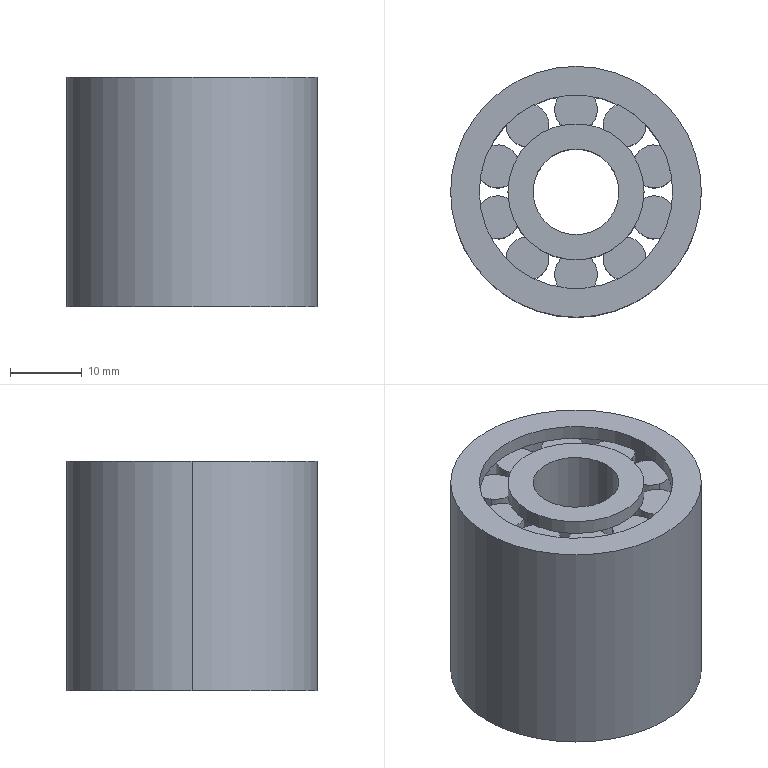Part | NX | features BREP 12 | 12 solids | 64 faces | box 35 x 35 x 32 mm | volume 21762 mm3 | cylinder 36 | plane 28 | commonest cylinder face diameters 6 x20 19 x4 27 x4 12 x2 17 x2 29 x2
STEP:
#1=CARTESIAN_POINT('',(-11.864,-0.7005,29.95));
#2=VERTEX_POINT('',#1);
#3=CARTESIAN_POINT('',(-10.01,-6.407,29.95));
#4=VERTEX_POINT('',#3);
#5=CARTESIAN_POINT('',(-10.937,-3.554,29.95));
#6=DIRECTION('',(0.,0.,1.));
#7=DIRECTION('',(-0.309,0.9511,0.));
#8=AXIS2_PLACEMENT_3D('',#5,#6,#7);
#9=CIRCLE('',#8,3.);
#10=EDGE_CURVE('',#2,#4,#9,.T.);
#11=ORIENTED_EDGE('',*,*,#10,.F.);
#12=CARTESIAN_POINT('',(-11.864,-0.7005,2.05));
#13=VERTEX_POINT('',#12);
#14=CARTESIAN_POINT('',(-11.864,-0.7005,29.95));
#15=DIRECTION('',(0.,0.,-1.));
#16=VECTOR('',#15,1000.);
#17=LINE('',#14,#16);
#18=EDGE_CURVE('',#2,#13,#17,.T.);
#19=ORIENTED_EDGE('',*,*,#18,.T.);
#20=CARTESIAN_POINT('',(-10.01,-6.407,2.05));
#21=VERTEX_POINT('',#20);
#22=CARTESIAN_POINT('',(-10.937,-3.554,2.05));
#23=DIRECTION('',(0.,0.,1.));
#24=DIRECTION('',(-0.309,0.9511,0.));
#25=AXIS2_PLACEMENT_3D('',#22,#23,#24);
#26=CIRCLE('',#25,3.);
#27=EDGE_CURVE('',#13,#21,#26,.T.);
#28=ORIENTED_EDGE('',*,*,#27,.T.);
#29=CARTESIAN_POINT('',(-10.01,-6.407,29.95));
#30=DIRECTION('',(0.,0.,-1.));
#31=VECTOR('',#30,1000.);
#32=LINE('',#29,#31);
#33=EDGE_CURVE('',#4,#21,#32,.T.);
#34=ORIENTED_EDGE('',*,*,#33,.F.);
#35=EDGE_LOOP('',(#11,#19,#28,#34));
#36=FACE_BOUND('',#35,.T.);
#37=CARTESIAN_POINT('',(-10.937,-3.554,29.95));
#38=DIRECTION('',(0.,0.,-1.));
#39=DIRECTION('',(-0.309,0.9511,0.));
#40=AXIS2_PLACEMENT_3D('',#37,#38,#39);
#41=CYLINDRICAL_SURFACE('',#40,3.);
#42=ADVANCED_FACE('',(#36),#41,.T.);
#43=ORIENTED_EDGE('',*,*,#18,.F.);
#44=CARTESIAN_POINT('',(-10.937,-3.554,29.95));
#45=DIRECTION('',(0.,0.,1.));
#46=DIRECTION('',(-0.309,0.9511,0.));
#47=AXIS2_PLACEMENT_3D('',#44,#45,#46);
#48=CIRCLE('',#47,3.);
#49=EDGE_CURVE('',#4,#2,#48,.T.);
#50=ORIENTED_EDGE('',*,*,#49,.F.);
#51=ORIENTED_EDGE('',*,*,#33,.T.);
#52=CARTESIAN_POINT('',(-10.937,-3.554,2.05));
#53=DIRECTION('',(0.,0.,1.));
#54=DIRECTION('',(-0.309,0.9511,0.));
#55=AXIS2_PLACEMENT_3D('',#52,#53,#54);
#56=CIRCLE('',#55,3.);
#57=EDGE_CURVE('',#21,#13,#56,.T.);
#58=ORIENTED_EDGE('',*,*,#57,.T.);
#59=EDGE_LOOP('',(#43,#50,#51,#58));
#60=FACE_BOUND('',#59,.T.);
#61=CARTESIAN_POINT('',(-10.937,-3.554,29.95));
#62=DIRECTION('',(0.,0.,-1.));
#63=DIRECTION('',(-0.309,0.9511,0.));
#64=AXIS2_PLACEMENT_3D('',#61,#62,#63);
#65=CYLINDRICAL_SURFACE('',#64,3.);
#66=ADVANCED_FACE('',(#60),#65,.T.);
#67=ORIENTED_EDGE('',*,*,#49,.T.);
#68=ORIENTED_EDGE('',*,*,#10,.T.);
#69=EDGE_LOOP('',(#67,#68));
#70=FACE_BOUND('',#69,.T.);
#71=CARTESIAN_POINT('',(-10.937,-3.554,29.95));
#72=DIRECTION('',(0.,0.,1.));
#73=DIRECTION('',(-1.,0.,0.));
#74=AXIS2_PLACEMENT_3D('',#71,#72,#73);
#75=PLANE('',#74);
#76=ADVANCED_FACE('',(#70),#75,.T.);
#77=ORIENTED_EDGE('',*,*,#57,.F.);
#78=ORIENTED_EDGE('',*,*,#27,.F.);
#79=EDGE_LOOP('',(#77,#78));
#80=FACE_BOUND('',#79,.T.);
#81=CARTESIAN_POINT('',(-10.937,-3.554,2.05));
#82=DIRECTION('',(0.,0.,1.));
#83=DIRECTION('',(-1.,0.,0.));
#84=AXIS2_PLACEMENT_3D('',#81,#82,#83);
#85=PLANE('',#84);
#86=ADVANCED_FACE('',(#80),#85,.F.);
#87=CLOSED_SHELL('',(#42,#66,#76,#86));
#88=MANIFOLD_SOLID_BREP('',#87);
#89=CARTESIAN_POINT('',(-4.332,11.067,29.95));
#90=VERTEX_POINT('',#89);
#91=CARTESIAN_POINT('',(-9.187,7.54,29.95));
#92=VERTEX_POINT('',#91);
#93=CARTESIAN_POINT('',(-6.76,9.304,29.95));
#94=DIRECTION('',(0.,0.,1.));
#95=DIRECTION('',(0.809,0.5878,0.));
#96=AXIS2_PLACEMENT_3D('',#93,#94,#95);
#97=CIRCLE('',#96,3.);
#98=EDGE_CURVE('',#90,#92,#97,.T.);
#99=ORIENTED_EDGE('',*,*,#98,.F.);
#100=CARTESIAN_POINT('',(-4.332,11.067,2.05));
#101=VERTEX_POINT('',#100);
#102=CARTESIAN_POINT('',(-4.332,11.067,29.95));
#103=DIRECTION('',(0.,0.,-1.));
#104=VECTOR('',#103,1000.);
#105=LINE('',#102,#104);
#106=EDGE_CURVE('',#101,#90,#105,.F.);
#107=ORIENTED_EDGE('',*,*,#106,.F.);
#108=CARTESIAN_POINT('',(-9.187,7.54,2.05));
#109=VERTEX_POINT('',#108);
#110=CARTESIAN_POINT('',(-6.76,9.304,2.05));
#111=DIRECTION('',(0.,0.,1.));
#112=DIRECTION('',(0.809,0.5878,0.));
#113=AXIS2_PLACEMENT_3D('',#110,#111,#112);
#114=CIRCLE('',#113,3.);
#115=EDGE_CURVE('',#101,#109,#114,.T.);
#116=ORIENTED_EDGE('',*,*,#115,.T.);
#117=CARTESIAN_POINT('',(-9.187,7.54,29.95));
#118=DIRECTION('',(0.,0.,-1.));
#119=VECTOR('',#118,1000.);
#120=LINE('',#117,#119);
#121=EDGE_CURVE('',#109,#92,#120,.F.);
#122=ORIENTED_EDGE('',*,*,#121,.T.);
#123=EDGE_LOOP('',(#99,#107,#116,#122));
#124=FACE_BOUND('',#123,.T.);
#125=CARTESIAN_POINT('',(-6.76,9.304,29.95));
#126=DIRECTION('',(0.,0.,-1.));
#127=DIRECTION('',(0.809,0.5878,0.));
#128=AXIS2_PLACEMENT_3D('',#125,#126,#127);
#129=CYLINDRICAL_SURFACE('',#128,3.);
#130=ADVANCED_FACE('',(#124),#129,.T.);
#131=ORIENTED_EDGE('',*,*,#106,.T.);
#132=CARTESIAN_POINT('',(-6.76,9.304,29.95));
#133=DIRECTION('',(0.,0.,1.));
#134=DIRECTION('',(0.809,0.5878,0.));
#135=AXIS2_PLACEMENT_3D('',#132,#133,#134);
#136=CIRCLE('',#135,3.);
#137=EDGE_CURVE('',#92,#90,#136,.T.);
#138=ORIENTED_EDGE('',*,*,#137,.F.);
#139=ORIENTED_EDGE('',*,*,#121,.F.);
#140=CARTESIAN_POINT('',(-6.76,9.304,2.05));
#141=DIRECTION('',(0.,0.,1.));
#142=DIRECTION('',(0.809,0.5878,0.));
#143=AXIS2_PLACEMENT_3D('',#140,#141,#142);
#144=CIRCLE('',#143,3.);
#145=EDGE_CURVE('',#109,#101,#144,.T.);
#146=ORIENTED_EDGE('',*,*,#145,.T.);
#147=EDGE_LOOP('',(#131,#138,#139,#146));
#148=FACE_BOUND('',#147,.T.);
#149=CARTESIAN_POINT('',(-6.76,9.304,29.95));
#150=DIRECTION('',(0.,0.,-1.));
#151=DIRECTION('',(0.809,0.5878,0.));
#152=AXIS2_PLACEMENT_3D('',#149,#150,#151);
#153=CYLINDRICAL_SURFACE('',#152,3.);
#154=ADVANCED_FACE('',(#148),#153,.T.);
#155=ORIENTED_EDGE('',*,*,#137,.T.);
#156=ORIENTED_EDGE('',*,*,#98,.T.);
#157=EDGE_LOOP('',(#155,#156));
#158=FACE_BOUND('',#157,.T.);
#159=CARTESIAN_POINT('',(-6.76,9.304,29.95));
#160=DIRECTION('',(0.,0.,1.));
#161=DIRECTION('',(-1.,0.,0.));
#162=AXIS2_PLACEMENT_3D('',#159,#160,#161);
#163=PLANE('',#162);
#164=ADVANCED_FACE('',(#158),#163,.T.);
#165=ORIENTED_EDGE('',*,*,#145,.F.);
#166=ORIENTED_EDGE('',*,*,#115,.F.);
#167=EDGE_LOOP('',(#165,#166));
#168=FACE_BOUND('',#167,.T.);
#169=CARTESIAN_POINT('',(-6.76,9.304,2.05));
#170=DIRECTION('',(0.,0.,1.));
#171=DIRECTION('',(-1.,0.,0.));
#172=AXIS2_PLACEMENT_3D('',#169,#170,#171);
#173=PLANE('',#172);
#174=ADVANCED_FACE('',(#168),#173,.F.);
#175=CLOSED_SHELL('',(#130,#154,#164,#174));
#176=MANIFOLD_SOLID_BREP('',#175);
#177=CARTESIAN_POINT('',(11.864,0.7005,29.95));
#178=VERTEX_POINT('',#177);
#179=CARTESIAN_POINT('',(10.01,6.407,29.95));
#180=VERTEX_POINT('',#179);
#181=CARTESIAN_POINT('',(10.937,3.554,29.95));
#182=DIRECTION('',(0.,0.,1.));
#183=DIRECTION('',(0.309,-0.9511,0.));
#184=AXIS2_PLACEMENT_3D('',#181,#182,#183);
#185=CIRCLE('',#184,3.);
#186=EDGE_CURVE('',#178,#180,#185,.T.);
#187=ORIENTED_EDGE('',*,*,#186,.F.);
#188=CARTESIAN_POINT('',(11.864,0.7005,2.05));
#189=VERTEX_POINT('',#188);
#190=CARTESIAN_POINT('',(11.864,0.7005,29.95));
#191=DIRECTION('',(0.,0.,-1.));
#192=VECTOR('',#191,1000.);
#193=LINE('',#190,#192);
#194=EDGE_CURVE('',#189,#178,#193,.F.);
#195=ORIENTED_EDGE('',*,*,#194,.F.);
#196=CARTESIAN_POINT('',(10.01,6.407,2.05));
#197=VERTEX_POINT('',#196);
#198=CARTESIAN_POINT('',(10.937,3.554,2.05));
#199=DIRECTION('',(0.,0.,1.));
#200=DIRECTION('',(0.309,-0.9511,0.));
#201=AXIS2_PLACEMENT_3D('',#198,#199,#200);
#202=CIRCLE('',#201,3.);
#203=EDGE_CURVE('',#189,#197,#202,.T.);
#204=ORIENTED_EDGE('',*,*,#203,.T.);
#205=CARTESIAN_POINT('',(10.01,6.407,29.95));
#206=DIRECTION('',(0.,0.,-1.));
#207=VECTOR('',#206,1000.);
#208=LINE('',#205,#207);
#209=EDGE_CURVE('',#197,#180,#208,.F.);
#210=ORIENTED_EDGE('',*,*,#209,.T.);
#211=EDGE_LOOP('',(#187,#195,#204,#210));
#212=FACE_BOUND('',#211,.T.);
#213=CARTESIAN_POINT('',(10.937,3.554,29.95));
#214=DIRECTION('',(0.,0.,-1.));
#215=DIRECTION('',(0.309,-0.9511,0.));
#216=AXIS2_PLACEMENT_3D('',#213,#214,#215);
#217=CYLINDRICAL_SURFACE('',#216,3.);
#218=ADVANCED_FACE('',(#212),#217,.T.);
#219=ORIENTED_EDGE('',*,*,#194,.T.);
#220=CARTESIAN_POINT('',(10.937,3.554,29.95));
#221=DIRECTION('',(0.,0.,1.));
#222=DIRECTION('',(0.309,-0.9511,0.));
#223=AXIS2_PLACEMENT_3D('',#220,#221,#222);
#224=CIRCLE('',#223,3.);
#225=EDGE_CURVE('',#180,#178,#224,.T.);
#226=ORIENTED_EDGE('',*,*,#225,.F.);
#227=ORIENTED_EDGE('',*,*,#209,.F.);
#228=CARTESIAN_POINT('',(10.937,3.554,2.05));
#229=DIRECTION('',(0.,0.,1.));
#230=DIRECTION('',(0.309,-0.9511,0.));
#231=AXIS2_PLACEMENT_3D('',#228,#229,#230);
#232=CIRCLE('',#231,3.);
#233=EDGE_CURVE('',#197,#189,#232,.T.);
#234=ORIENTED_EDGE('',*,*,#233,.T.);
#235=EDGE_LOOP('',(#219,#226,#227,#234));
#236=FACE_BOUND('',#235,.T.);
#237=CARTESIAN_POINT('',(10.937,3.554,29.95));
#238=DIRECTION('',(0.,0.,-1.));
#239=DIRECTION('',(0.309,-0.9511,0.));
#240=AXIS2_PLACEMENT_3D('',#237,#238,#239);
#241=CYLINDRICAL_SURFACE('',#240,3.);
#242=ADVANCED_FACE('',(#236),#241,.T.);
#243=ORIENTED_EDGE('',*,*,#225,.T.);
#244=ORIENTED_EDGE('',*,*,#186,.T.);
#245=EDGE_LOOP('',(#243,#244));
#246=FACE_BOUND('',#245,.T.);
#247=CARTESIAN_POINT('',(10.937,3.554,29.95));
#248=DIRECTION('',(0.,0.,1.));
#249=DIRECTION('',(-1.,0.,0.));
#250=AXIS2_PLACEMENT_3D('',#247,#248,#249);
#251=PLANE('',#250);
#252=ADVANCED_FACE('',(#246),#251,.T.);
#253=ORIENTED_EDGE('',*,*,#233,.F.);
#254=ORIENTED_EDGE('',*,*,#203,.F.);
#255=EDGE_LOOP('',(#253,#254));
#256=FACE_BOUND('',#255,.T.);
#257=CARTESIAN_POINT('',(10.937,3.554,2.05));
#258=DIRECTION('',(0.,0.,1.));
#259=DIRECTION('',(-1.,0.,0.));
#260=AXIS2_PLACEMENT_3D('',#257,#258,#259);
#261=PLANE('',#260);
#262=ADVANCED_FACE('',(#256),#261,.F.);
#263=CLOSED_SHELL('',(#218,#242,#252,#262));
#264=MANIFOLD_SOLID_BREP('',#263);
#265=CARTESIAN_POINT('',(8.5,0.,2.));
#266=VERTEX_POINT('',#265);
#267=CARTESIAN_POINT('',(-8.5,0.,2.));
#268=VERTEX_POINT('',#267);
#269=CARTESIAN_POINT('',(0.,0.,2.));
#270=DIRECTION('',(0.,0.,1.));
#271=DIRECTION('',(1.,0.,0.));
#272=AXIS2_PLACEMENT_3D('',#269,#270,#271);
#273=CIRCLE('',#272,8.5);
#274=EDGE_CURVE('',#266,#268,#273,.T.);
#275=ORIENTED_EDGE('',*,*,#274,.T.);
#276=CARTESIAN_POINT('',(-8.5,0.,30.));
#277=VERTEX_POINT('',#276);
#278=CARTESIAN_POINT('',(-8.5,0.,32.));
#279=DIRECTION('',(0.,0.,1.));
#280=VECTOR('',#279,1000.);
#281=LINE('',#278,#280);
#282=EDGE_CURVE('',#268,#277,#281,.T.);
#283=ORIENTED_EDGE('',*,*,#282,.T.);
#284=CARTESIAN_POINT('',(8.5,0.,30.));
#285=VERTEX_POINT('',#284);
#286=CARTESIAN_POINT('',(0.,0.,30.));
#287=DIRECTION('',(0.,0.,1.));
#288=DIRECTION('',(1.,0.,0.));
#289=AXIS2_PLACEMENT_3D('',#286,#287,#288);
#290=CIRCLE('',#289,8.5);
#291=EDGE_CURVE('',#285,#277,#290,.T.);
#292=ORIENTED_EDGE('',*,*,#291,.F.);
#293=CARTESIAN_POINT('',(8.5,0.,32.));
#294=DIRECTION('',(0.,0.,1.));
#295=VECTOR('',#294,1000.);
#296=LINE('',#293,#295);
#297=EDGE_CURVE('',#266,#285,#296,.T.);
#298=ORIENTED_EDGE('',*,*,#297,.F.);
#299=EDGE_LOOP('',(#275,#283,#292,#298));
#300=FACE_BOUND('',#299,.T.);
#301=CARTESIAN_POINT('',(0.,0.,32.));
#302=DIRECTION('',(0.,0.,1.));
#303=DIRECTION('',(-1.,0.,0.));
#304=AXIS2_PLACEMENT_3D('',#301,#302,#303);
#305=CYLINDRICAL_SURFACE('',#304,8.5);
#306=ADVANCED_FACE('',(#300),#305,.T.);
#307=CARTESIAN_POINT('',(-6.,0.,32.));
#308=VERTEX_POINT('',#307);
#309=CARTESIAN_POINT('',(6.,0.,32.));
#310=VERTEX_POINT('',#309);
#311=CARTESIAN_POINT('',(0.,0.,32.));
#312=DIRECTION('',(0.,0.,1.));
#313=DIRECTION('',(1.,0.,0.));
#314=AXIS2_PLACEMENT_3D('',#311,#312,#313);
#315=CIRCLE('',#314,6.);
#316=EDGE_CURVE('',#308,#310,#315,.T.);
#317=ORIENTED_EDGE('',*,*,#316,.T.);
#318=CARTESIAN_POINT('',(6.,0.,0.));
#319=VERTEX_POINT('',#318);
#320=CARTESIAN_POINT('',(6.,0.,32.));
#321=DIRECTION('',(0.,0.,-1.));
#322=VECTOR('',#321,1000.);
#323=LINE('',#320,#322);
#324=EDGE_CURVE('',#319,#310,#323,.F.);
#325=ORIENTED_EDGE('',*,*,#324,.F.);
#326=CARTESIAN_POINT('',(-6.,0.,0.));
#327=VERTEX_POINT('',#326);
#328=CARTESIAN_POINT('',(0.,0.,0.));
#329=DIRECTION('',(0.,0.,1.));
#330=DIRECTION('',(1.,0.,0.));
#331=AXIS2_PLACEMENT_3D('',#328,#329,#330);
#332=CIRCLE('',#331,6.);
#333=EDGE_CURVE('',#327,#319,#332,.T.);
#334=ORIENTED_EDGE('',*,*,#333,.F.);
#335=CARTESIAN_POINT('',(-6.,0.,32.));
#336=DIRECTION('',(0.,0.,-1.));
#337=VECTOR('',#336,1000.);
#338=LINE('',#335,#337);
#339=EDGE_CURVE('',#327,#308,#338,.F.);
#340=ORIENTED_EDGE('',*,*,#339,.T.);
#341=EDGE_LOOP('',(#317,#325,#334,#340));
#342=FACE_BOUND('',#341,.T.);
#343=CARTESIAN_POINT('',(0.,0.,32.));
#344=DIRECTION('',(0.,0.,-1.));
#345=DIRECTION('',(1.,0.,0.));
#346=AXIS2_PLACEMENT_3D('',#343,#344,#345);
#347=CYLINDRICAL_SURFACE('',#346,6.);
#348=ADVANCED_FACE('',(#342),#347,.F.);
#349=CARTESIAN_POINT('',(9.5,0.,2.));
#350=VERTEX_POINT('',#349);
#351=CARTESIAN_POINT('',(-9.5,0.,2.));
#352=VERTEX_POINT('',#351);
#353=CARTESIAN_POINT('',(0.,0.,2.));
#354=DIRECTION('',(0.,0.,1.));
#355=DIRECTION('',(1.,0.,0.));
#356=AXIS2_PLACEMENT_3D('',#353,#354,#355);
#357=CIRCLE('',#356,9.5);
#358=EDGE_CURVE('',#350,#352,#357,.T.);
#359=ORIENTED_EDGE('',*,*,#358,.F.);
#360=CARTESIAN_POINT('',(9.5,0.,0.));
#361=VERTEX_POINT('',#360);
#362=CARTESIAN_POINT('',(9.5,0.,32.));
#363=DIRECTION('',(0.,0.,-1.));
#364=VECTOR('',#363,1000.);
#365=LINE('',#362,#364);
#366=EDGE_CURVE('',#361,#350,#365,.F.);
#367=ORIENTED_EDGE('',*,*,#366,.F.);
#368=CARTESIAN_POINT('',(-9.5,0.,0.));
#369=VERTEX_POINT('',#368);
#370=CARTESIAN_POINT('',(0.,0.,0.));
#371=DIRECTION('',(0.,0.,1.));
#372=DIRECTION('',(1.,0.,0.));
#373=AXIS2_PLACEMENT_3D('',#370,#371,#372);
#374=CIRCLE('',#373,9.5);
#375=EDGE_CURVE('',#361,#369,#374,.T.);
#376=ORIENTED_EDGE('',*,*,#375,.T.);
#377=CARTESIAN_POINT('',(-9.5,0.,32.));
#378=DIRECTION('',(0.,0.,-1.));
#379=VECTOR('',#378,1000.);
#380=LINE('',#377,#379);
#381=EDGE_CURVE('',#369,#352,#380,.F.);
#382=ORIENTED_EDGE('',*,*,#381,.T.);
#383=EDGE_LOOP('',(#359,#367,#376,#382));
#384=FACE_BOUND('',#383,.T.);
#385=CARTESIAN_POINT('',(0.,0.,32.));
#386=DIRECTION('',(0.,0.,-1.));
#387=DIRECTION('',(1.,0.,0.));
#388=AXIS2_PLACEMENT_3D('',#385,#386,#387);
#389=CYLINDRICAL_SURFACE('',#388,9.5);
#390=ADVANCED_FACE('',(#384),#389,.T.);
#391=CARTESIAN_POINT('',(9.5,0.,32.));
#392=VERTEX_POINT('',#391);
#393=CARTESIAN_POINT('',(-9.5,0.,32.));
#394=VERTEX_POINT('',#393);
#395=CARTESIAN_POINT('',(0.,0.,32.));
#396=DIRECTION('',(0.,0.,1.));
#397=DIRECTION('',(1.,0.,0.));
#398=AXIS2_PLACEMENT_3D('',#395,#396,#397);
#399=CIRCLE('',#398,9.5);
#400=EDGE_CURVE('',#392,#394,#399,.T.);
#401=ORIENTED_EDGE('',*,*,#400,.F.);
#402=CARTESIAN_POINT('',(9.5,0.,30.));
#403=VERTEX_POINT('',#402);
#404=CARTESIAN_POINT('',(9.5,0.,32.));
#405=DIRECTION('',(0.,0.,-1.));
#406=VECTOR('',#405,1000.);
#407=LINE('',#404,#406);
#408=EDGE_CURVE('',#403,#392,#407,.F.);
#409=ORIENTED_EDGE('',*,*,#408,.F.);
#410=CARTESIAN_POINT('',(-9.5,0.,30.));
#411=VERTEX_POINT('',#410);
#412=CARTESIAN_POINT('',(0.,0.,30.));
#413=DIRECTION('',(0.,0.,-1.));
#414=DIRECTION('',(-1.,0.,0.));
#415=AXIS2_PLACEMENT_3D('',#412,#413,#414);
#416=CIRCLE('',#415,9.5);
#417=EDGE_CURVE('',#411,#403,#416,.T.);
#418=ORIENTED_EDGE('',*,*,#417,.F.);
#419=CARTESIAN_POINT('',(-9.5,0.,32.));
#420=DIRECTION('',(0.,0.,-1.));
#421=VECTOR('',#420,1000.);
#422=LINE('',#419,#421);
#423=EDGE_CURVE('',#411,#394,#422,.F.);
#424=ORIENTED_EDGE('',*,*,#423,.T.);
#425=EDGE_LOOP('',(#401,#409,#418,#424));
#426=FACE_BOUND('',#425,.T.);
#427=CARTESIAN_POINT('',(0.,0.,32.));
#428=DIRECTION('',(0.,0.,-1.));
#429=DIRECTION('',(1.,0.,0.));
#430=AXIS2_PLACEMENT_3D('',#427,#428,#429);
#431=CYLINDRICAL_SURFACE('',#430,9.5);
#432=ADVANCED_FACE('',(#426),#431,.T.);
#433=ORIENTED_EDGE('',*,*,#408,.T.);
#434=CARTESIAN_POINT('',(0.,0.,32.));
#435=DIRECTION('',(0.,0.,1.));
#436=DIRECTION('',(1.,0.,0.));
#437=AXIS2_PLACEMENT_3D('',#434,#435,#436);
#438=CIRCLE('',#437,9.5);
#439=EDGE_CURVE('',#394,#392,#438,.T.);
#440=ORIENTED_EDGE('',*,*,#439,.F.);
#441=ORIENTED_EDGE('',*,*,#423,.F.);
#442=CARTESIAN_POINT('',(0.,0.,30.));
#443=DIRECTION('',(0.,0.,-1.));
#444=DIRECTION('',(-1.,0.,0.));
#445=AXIS2_PLACEMENT_3D('',#442,#443,#444);
#446=CIRCLE('',#445,9.5);
#447=EDGE_CURVE('',#403,#411,#446,.T.);
#448=ORIENTED_EDGE('',*,*,#447,.F.);
#449=EDGE_LOOP('',(#433,#440,#441,#448));
#450=FACE_BOUND('',#449,.T.);
#451=CARTESIAN_POINT('',(0.,0.,32.));
#452=DIRECTION('',(0.,0.,-1.));
#453=DIRECTION('',(1.,0.,0.));
#454=AXIS2_PLACEMENT_3D('',#451,#452,#453);
#455=CYLINDRICAL_SURFACE('',#454,9.5);
#456=ADVANCED_FACE('',(#450),#455,.T.);
#457=ORIENTED_EDGE('',*,*,#366,.T.);
#458=CARTESIAN_POINT('',(0.,0.,2.));
#459=DIRECTION('',(0.,0.,1.));
#460=DIRECTION('',(1.,0.,0.));
#461=AXIS2_PLACEMENT_3D('',#458,#459,#460);
#462=CIRCLE('',#461,9.5);
#463=EDGE_CURVE('',#352,#350,#462,.T.);
#464=ORIENTED_EDGE('',*,*,#463,.F.);
#465=ORIENTED_EDGE('',*,*,#381,.F.);
#466=CARTESIAN_POINT('',(0.,0.,0.));
#467=DIRECTION('',(0.,0.,1.));
#468=DIRECTION('',(1.,0.,0.));
#469=AXIS2_PLACEMENT_3D('',#466,#467,#468);
#470=CIRCLE('',#469,9.5);
#471=EDGE_CURVE('',#369,#361,#470,.T.);
#472=ORIENTED_EDGE('',*,*,#471,.T.);
#473=EDGE_LOOP('',(#457,#464,#465,#472));
#474=FACE_BOUND('',#473,.T.);
#475=CARTESIAN_POINT('',(0.,0.,32.));
#476=DIRECTION('',(0.,0.,-1.));
#477=DIRECTION('',(1.,0.,0.));
#478=AXIS2_PLACEMENT_3D('',#475,#476,#477);
#479=CYLINDRICAL_SURFACE('',#478,9.5);
#480=ADVANCED_FACE('',(#474),#479,.T.);
#481=ORIENTED_EDGE('',*,*,#324,.T.);
#482=CARTESIAN_POINT('',(0.,0.,32.));
#483=DIRECTION('',(0.,0.,1.));
#484=DIRECTION('',(1.,0.,0.));
#485=AXIS2_PLACEMENT_3D('',#482,#483,#484);
#486=CIRCLE('',#485,6.);
#487=EDGE_CURVE('',#310,#308,#486,.T.);
#488=ORIENTED_EDGE('',*,*,#487,.T.);
#489=ORIENTED_EDGE('',*,*,#339,.F.);
#490=CARTESIAN_POINT('',(0.,0.,0.));
#491=DIRECTION('',(0.,0.,1.));
#492=DIRECTION('',(1.,0.,0.));
#493=AXIS2_PLACEMENT_3D('',#490,#491,#492);
#494=CIRCLE('',#493,6.);
#495=EDGE_CURVE('',#319,#327,#494,.T.);
#496=ORIENTED_EDGE('',*,*,#495,.F.);
#497=EDGE_LOOP('',(#481,#488,#489,#496));
#498=FACE_BOUND('',#497,.T.);
#499=CARTESIAN_POINT('',(0.,0.,32.));
#500=DIRECTION('',(0.,0.,-1.));
#501=DIRECTION('',(1.,0.,0.));
#502=AXIS2_PLACEMENT_3D('',#499,#500,#501);
#503=CYLINDRICAL_SURFACE('',#502,6.);
#504=ADVANCED_FACE('',(#498),#503,.F.);
#505=ORIENTED_EDGE('',*,*,#439,.T.);
#506=ORIENTED_EDGE('',*,*,#400,.T.);
#507=EDGE_LOOP('',(#505,#506));
#508=FACE_BOUND('',#507,.T.);
#509=ORIENTED_EDGE('',*,*,#316,.F.);
#510=ORIENTED_EDGE('',*,*,#487,.F.);
#511=EDGE_LOOP('',(#509,#510));
#512=FACE_BOUND('',#511,.T.);
#513=CARTESIAN_POINT('',(0.,0.,32.));
#514=DIRECTION('',(0.,0.,1.));
#515=DIRECTION('',(-1.,0.,0.));
#516=AXIS2_PLACEMENT_3D('',#513,#514,#515);
#517=PLANE('',#516);
#518=ADVANCED_FACE('',(#508,#512),#517,.T.);
#519=ORIENTED_EDGE('',*,*,#471,.F.);
#520=ORIENTED_EDGE('',*,*,#375,.F.);
#521=EDGE_LOOP('',(#519,#520));
#522=FACE_BOUND('',#521,.T.);
#523=ORIENTED_EDGE('',*,*,#333,.T.);
#524=ORIENTED_EDGE('',*,*,#495,.T.);
#525=EDGE_LOOP('',(#523,#524));
#526=FACE_BOUND('',#525,.T.);
#527=CARTESIAN_POINT('',(0.,0.,0.));
#528=DIRECTION('',(0.,0.,1.));
#529=DIRECTION('',(-1.,0.,0.));
#530=AXIS2_PLACEMENT_3D('',#527,#528,#529);
#531=PLANE('',#530);
#532=ADVANCED_FACE('',(#522,#526),#531,.F.);
#533=ORIENTED_EDGE('',*,*,#417,.T.);
#534=ORIENTED_EDGE('',*,*,#447,.T.);
#535=EDGE_LOOP('',(#533,#534));
#536=FACE_BOUND('',#535,.T.);
#537=ORIENTED_EDGE('',*,*,#291,.T.);
#538=CARTESIAN_POINT('',(0.,0.,30.));
#539=DIRECTION('',(0.,0.,1.));
#540=DIRECTION('',(1.,0.,0.));
#541=AXIS2_PLACEMENT_3D('',#538,#539,#540);
#542=CIRCLE('',#541,8.5);
#543=EDGE_CURVE('',#277,#285,#542,.T.);
#544=ORIENTED_EDGE('',*,*,#543,.T.);
#545=EDGE_LOOP('',(#537,#544));
#546=FACE_BOUND('',#545,.T.);
#547=CARTESIAN_POINT('',(0.,14.5,30.));
#548=DIRECTION('',(0.,0.,-1.));
#549=DIRECTION('',(0.,1.,0.));
#550=AXIS2_PLACEMENT_3D('',#547,#548,#549);
#551=PLANE('',#550);
#552=ADVANCED_FACE('',(#536,#546),#551,.T.);
#553=ORIENTED_EDGE('',*,*,#463,.T.);
#554=ORIENTED_EDGE('',*,*,#358,.T.);
#555=EDGE_LOOP('',(#553,#554));
#556=FACE_BOUND('',#555,.T.);
#557=ORIENTED_EDGE('',*,*,#274,.F.);
#558=CARTESIAN_POINT('',(0.,0.,2.));
#559=DIRECTION('',(0.,0.,1.));
#560=DIRECTION('',(1.,0.,0.));
#561=AXIS2_PLACEMENT_3D('',#558,#559,#560);
#562=CIRCLE('',#561,8.5);
#563=EDGE_CURVE('',#268,#266,#562,.T.);
#564=ORIENTED_EDGE('',*,*,#563,.F.);
#565=EDGE_LOOP('',(#557,#564));
#566=FACE_BOUND('',#565,.T.);
#567=CARTESIAN_POINT('',(0.,14.5,2.));
#568=DIRECTION('',(0.,0.,1.));
#569=DIRECTION('',(-1.,0.,0.));
#570=AXIS2_PLACEMENT_3D('',#567,#568,#569);
#571=PLANE('',#570);
#572=ADVANCED_FACE('',(#556,#566),#571,.T.);
#573=ORIENTED_EDGE('',*,*,#282,.F.);
#574=ORIENTED_EDGE('',*,*,#563,.T.);
#575=ORIENTED_EDGE('',*,*,#297,.T.);
#576=ORIENTED_EDGE('',*,*,#543,.F.);
#577=EDGE_LOOP('',(#573,#574,#575,#576));
#578=FACE_BOUND('',#577,.T.);
#579=CARTESIAN_POINT('',(0.,0.,32.));
#580=DIRECTION('',(0.,0.,1.));
#581=DIRECTION('',(-1.,0.,0.));
#582=AXIS2_PLACEMENT_3D('',#579,#580,#581);
#583=CYLINDRICAL_SURFACE('',#582,8.5);
#584=ADVANCED_FACE('',(#578),#583,.T.);
#585=CLOSED_SHELL('',(#306,#348,#390,#432,#456,#480,#504,#518,#532,#552,#572,#584));
#586=MANIFOLD_SOLID_BREP('',#585);
#587=CARTESIAN_POINT('',(4.332,-11.067,29.95));
#588=VERTEX_POINT('',#587);
#589=CARTESIAN_POINT('',(9.187,-7.54,29.95));
#590=VERTEX_POINT('',#589);
#591=CARTESIAN_POINT('',(6.76,-9.304,29.95));
#592=DIRECTION('',(0.,0.,1.));
#593=DIRECTION('',(-0.809,-0.5878,0.));
#594=AXIS2_PLACEMENT_3D('',#591,#592,#593);
#595=CIRCLE('',#594,3.);
#596=EDGE_CURVE('',#588,#590,#595,.T.);
#597=ORIENTED_EDGE('',*,*,#596,.F.);
#598=CARTESIAN_POINT('',(4.332,-11.067,2.05));
#599=VERTEX_POINT('',#598);
#600=CARTESIAN_POINT('',(4.332,-11.067,29.95));
#601=DIRECTION('',(0.,0.,-1.));
#602=VECTOR('',#601,1000.);
#603=LINE('',#600,#602);
#604=EDGE_CURVE('',#588,#599,#603,.T.);
#605=ORIENTED_EDGE('',*,*,#604,.T.);
#606=CARTESIAN_POINT('',(9.187,-7.54,2.05));
#607=VERTEX_POINT('',#606);
#608=CARTESIAN_POINT('',(6.76,-9.304,2.05));
#609=DIRECTION('',(0.,0.,1.));
#610=DIRECTION('',(-0.809,-0.5878,0.));
#611=AXIS2_PLACEMENT_3D('',#608,#609,#610);
#612=CIRCLE('',#611,3.);
#613=EDGE_CURVE('',#599,#607,#612,.T.);
#614=ORIENTED_EDGE('',*,*,#613,.T.);
#615=CARTESIAN_POINT('',(9.187,-7.54,29.95));
#616=DIRECTION('',(0.,0.,-1.));
#617=VECTOR('',#616,1000.);
#618=LINE('',#615,#617);
#619=EDGE_CURVE('',#590,#607,#618,.T.);
#620=ORIENTED_EDGE('',*,*,#619,.F.);
#621=EDGE_LOOP('',(#597,#605,#614,#620));
#622=FACE_BOUND('',#621,.T.);
#623=CARTESIAN_POINT('',(6.76,-9.304,29.95));
#624=DIRECTION('',(0.,0.,-1.));
#625=DIRECTION('',(-0.809,-0.5878,0.));
#626=AXIS2_PLACEMENT_3D('',#623,#624,#625);
#627=CYLINDRICAL_SURFACE('',#626,3.);
#628=ADVANCED_FACE('',(#622),#627,.T.);
#629=ORIENTED_EDGE('',*,*,#604,.F.);
#630=CARTESIAN_POINT('',(6.76,-9.304,29.95));
#631=DIRECTION('',(0.,0.,1.));
#632=DIRECTION('',(-0.809,-0.5878,0.));
#633=AXIS2_PLACEMENT_3D('',#630,#631,#632);
#634=CIRCLE('',#633,3.);
#635=EDGE_CURVE('',#590,#588,#634,.T.);
#636=ORIENTED_EDGE('',*,*,#635,.F.);
#637=ORIENTED_EDGE('',*,*,#619,.T.);
#638=CARTESIAN_POINT('',(6.76,-9.304,2.05));
#639=DIRECTION('',(0.,0.,1.));
#640=DIRECTION('',(-0.809,-0.5878,0.));
#641=AXIS2_PLACEMENT_3D('',#638,#639,#640);
#642=CIRCLE('',#641,3.);
#643=EDGE_CURVE('',#607,#599,#642,.T.);
#644=ORIENTED_EDGE('',*,*,#643,.T.);
#645=EDGE_LOOP('',(#629,#636,#637,#644));
#646=FACE_BOUND('',#645,.T.);
#647=CARTESIAN_POINT('',(6.76,-9.304,29.95));
#648=DIRECTION('',(0.,0.,-1.));
#649=DIRECTION('',(-0.809,-0.5878,0.));
#650=AXIS2_PLACEMENT_3D('',#647,#648,#649);
#651=CYLINDRICAL_SURFACE('',#650,3.);
#652=ADVANCED_FACE('',(#646),#651,.T.);
#653=ORIENTED_EDGE('',*,*,#635,.T.);
#654=ORIENTED_EDGE('',*,*,#596,.T.);
#655=EDGE_LOOP('',(#653,#654));
#656=FACE_BOUND('',#655,.T.);
#657=CARTESIAN_POINT('',(6.76,-9.304,29.95));
#658=DIRECTION('',(0.,0.,1.));
#659=DIRECTION('',(-1.,0.,0.));
#660=AXIS2_PLACEMENT_3D('',#657,#658,#659);
#661=PLANE('',#660);
#662=ADVANCED_FACE('',(#656),#661,.T.);
#663=ORIENTED_EDGE('',*,*,#643,.F.);
#664=ORIENTED_EDGE('',*,*,#613,.F.);
#665=EDGE_LOOP('',(#663,#664));
#666=FACE_BOUND('',#665,.T.);
#667=CARTESIAN_POINT('',(6.76,-9.304,2.05));
#668=DIRECTION('',(0.,0.,1.));
#669=DIRECTION('',(-1.,0.,0.));
#670=AXIS2_PLACEMENT_3D('',#667,#668,#669);
#671=PLANE('',#670);
#672=ADVANCED_FACE('',(#666),#671,.F.);
#673=CLOSED_SHELL('',(#628,#652,#662,#672));
#674=MANIFOLD_SOLID_BREP('',#673);
#675=CARTESIAN_POINT('',(-9.187,-7.54,29.95));
#676=VERTEX_POINT('',#675);
#677=CARTESIAN_POINT('',(-4.332,-11.067,29.95));
#678=VERTEX_POINT('',#677);
#679=CARTESIAN_POINT('',(-6.76,-9.304,29.95));
#680=DIRECTION('',(0.,0.,1.));
#681=DIRECTION('',(-0.809,0.5878,0.));
#682=AXIS2_PLACEMENT_3D('',#679,#680,#681);
#683=CIRCLE('',#682,3.);
#684=EDGE_CURVE('',#676,#678,#683,.T.);
#685=ORIENTED_EDGE('',*,*,#684,.F.);
#686=CARTESIAN_POINT('',(-9.187,-7.54,2.05));
#687=VERTEX_POINT('',#686);
#688=CARTESIAN_POINT('',(-9.187,-7.54,29.95));
#689=DIRECTION('',(0.,0.,-1.));
#690=VECTOR('',#689,1000.);
#691=LINE('',#688,#690);
#692=EDGE_CURVE('',#676,#687,#691,.T.);
#693=ORIENTED_EDGE('',*,*,#692,.T.);
#694=CARTESIAN_POINT('',(-4.332,-11.067,2.05));
#695=VERTEX_POINT('',#694);
#696=CARTESIAN_POINT('',(-6.76,-9.304,2.05));
#697=DIRECTION('',(0.,0.,1.));
#698=DIRECTION('',(-0.809,0.5878,0.));
#699=AXIS2_PLACEMENT_3D('',#696,#697,#698);
#700=CIRCLE('',#699,3.);
#701=EDGE_CURVE('',#687,#695,#700,.T.);
#702=ORIENTED_EDGE('',*,*,#701,.T.);
#703=CARTESIAN_POINT('',(-4.332,-11.067,29.95));
#704=DIRECTION('',(0.,0.,-1.));
#705=VECTOR('',#704,1000.);
#706=LINE('',#703,#705);
#707=EDGE_CURVE('',#678,#695,#706,.T.);
#708=ORIENTED_EDGE('',*,*,#707,.F.);
#709=EDGE_LOOP('',(#685,#693,#702,#708));
#710=FACE_BOUND('',#709,.T.);
#711=CARTESIAN_POINT('',(-6.76,-9.304,29.95));
#712=DIRECTION('',(0.,0.,-1.));
#713=DIRECTION('',(-0.809,0.5878,0.));
#714=AXIS2_PLACEMENT_3D('',#711,#712,#713);
#715=CYLINDRICAL_SURFACE('',#714,3.);
#716=ADVANCED_FACE('',(#710),#715,.T.);
#717=ORIENTED_EDGE('',*,*,#692,.F.);
#718=CARTESIAN_POINT('',(-6.76,-9.304,29.95));
#719=DIRECTION('',(0.,0.,1.));
#720=DIRECTION('',(-0.809,0.5878,0.));
#721=AXIS2_PLACEMENT_3D('',#718,#719,#720);
#722=CIRCLE('',#721,3.);
#723=EDGE_CURVE('',#678,#676,#722,.T.);
#724=ORIENTED_EDGE('',*,*,#723,.F.);
#725=ORIENTED_EDGE('',*,*,#707,.T.);
#726=CARTESIAN_POINT('',(-6.76,-9.304,2.05));
#727=DIRECTION('',(0.,0.,1.));
#728=DIRECTION('',(-0.809,0.5878,0.));
#729=AXIS2_PLACEMENT_3D('',#726,#727,#728);
#730=CIRCLE('',#729,3.);
#731=EDGE_CURVE('',#695,#687,#730,.T.);
#732=ORIENTED_EDGE('',*,*,#731,.T.);
#733=EDGE_LOOP('',(#717,#724,#725,#732));
#734=FACE_BOUND('',#733,.T.);
#735=CARTESIAN_POINT('',(-6.76,-9.304,29.95));
#736=DIRECTION('',(0.,0.,-1.));
#737=DIRECTION('',(-0.809,0.5878,0.));
#738=AXIS2_PLACEMENT_3D('',#735,#736,#737);
#739=CYLINDRICAL_SURFACE('',#738,3.);
#740=ADVANCED_FACE('',(#734),#739,.T.);
#741=ORIENTED_EDGE('',*,*,#723,.T.);
#742=ORIENTED_EDGE('',*,*,#684,.T.);
#743=EDGE_LOOP('',(#741,#742));
#744=FACE_BOUND('',#743,.T.);
#745=CARTESIAN_POINT('',(-6.76,-9.304,29.95));
#746=DIRECTION('',(0.,0.,1.));
#747=DIRECTION('',(-1.,0.,0.));
#748=AXIS2_PLACEMENT_3D('',#745,#746,#747);
#749=PLANE('',#748);
#750=ADVANCED_FACE('',(#744),#749,.T.);
#751=ORIENTED_EDGE('',*,*,#731,.F.);
#752=ORIENTED_EDGE('',*,*,#701,.F.);
#753=EDGE_LOOP('',(#751,#752));
#754=FACE_BOUND('',#753,.T.);
#755=CARTESIAN_POINT('',(-6.76,-9.304,2.05));
#756=DIRECTION('',(0.,0.,1.));
#757=DIRECTION('',(-1.,0.,0.));
#758=AXIS2_PLACEMENT_3D('',#755,#756,#757);
#759=PLANE('',#758);
#760=ADVANCED_FACE('',(#754),#759,.F.);
#761=CLOSED_SHELL('',(#716,#740,#750,#760));
#762=MANIFOLD_SOLID_BREP('',#761);
#763=CARTESIAN_POINT('',(-10.01,6.407,29.95));
#764=VERTEX_POINT('',#763);
#765=CARTESIAN_POINT('',(-11.864,0.7005,29.95));
#766=VERTEX_POINT('',#765);
#767=CARTESIAN_POINT('',(-10.937,3.554,29.95));
#768=DIRECTION('',(0.,0.,1.));
#769=DIRECTION('',(0.309,0.9511,0.));
#770=AXIS2_PLACEMENT_3D('',#767,#768,#769);
#771=CIRCLE('',#770,3.);
#772=EDGE_CURVE('',#764,#766,#771,.T.);
#773=ORIENTED_EDGE('',*,*,#772,.F.);
#774=CARTESIAN_POINT('',(-10.01,6.407,2.05));
#775=VERTEX_POINT('',#774);
#776=CARTESIAN_POINT('',(-10.01,6.407,29.95));
#777=DIRECTION('',(0.,0.,-1.));
#778=VECTOR('',#777,1000.);
#779=LINE('',#776,#778);
#780=EDGE_CURVE('',#775,#764,#779,.F.);
#781=ORIENTED_EDGE('',*,*,#780,.F.);
#782=CARTESIAN_POINT('',(-11.864,0.7005,2.05));
#783=VERTEX_POINT('',#782);
#784=CARTESIAN_POINT('',(-10.937,3.554,2.05));
#785=DIRECTION('',(0.,0.,1.));
#786=DIRECTION('',(0.309,0.9511,0.));
#787=AXIS2_PLACEMENT_3D('',#784,#785,#786);
#788=CIRCLE('',#787,3.);
#789=EDGE_CURVE('',#775,#783,#788,.T.);
#790=ORIENTED_EDGE('',*,*,#789,.T.);
#791=CARTESIAN_POINT('',(-11.864,0.7005,29.95));
#792=DIRECTION('',(0.,0.,-1.));
#793=VECTOR('',#792,1000.);
#794=LINE('',#791,#793);
#795=EDGE_CURVE('',#783,#766,#794,.F.);
#796=ORIENTED_EDGE('',*,*,#795,.T.);
#797=EDGE_LOOP('',(#773,#781,#790,#796));
#798=FACE_BOUND('',#797,.T.);
#799=CARTESIAN_POINT('',(-10.937,3.554,29.95));
#800=DIRECTION('',(0.,0.,-1.));
#801=DIRECTION('',(0.309,0.9511,0.));
#802=AXIS2_PLACEMENT_3D('',#799,#800,#801);
#803=CYLINDRICAL_SURFACE('',#802,3.);
#804=ADVANCED_FACE('',(#798),#803,.T.);
#805=ORIENTED_EDGE('',*,*,#780,.T.);
#806=CARTESIAN_POINT('',(-10.937,3.554,29.95));
#807=DIRECTION('',(0.,0.,1.));
#808=DIRECTION('',(0.309,0.9511,0.));
#809=AXIS2_PLACEMENT_3D('',#806,#807,#808);
#810=CIRCLE('',#809,3.);
#811=EDGE_CURVE('',#766,#764,#810,.T.);
#812=ORIENTED_EDGE('',*,*,#811,.F.);
#813=ORIENTED_EDGE('',*,*,#795,.F.);
#814=CARTESIAN_POINT('',(-10.937,3.554,2.05));
#815=DIRECTION('',(0.,0.,1.));
#816=DIRECTION('',(0.309,0.9511,0.));
#817=AXIS2_PLACEMENT_3D('',#814,#815,#816);
#818=CIRCLE('',#817,3.);
#819=EDGE_CURVE('',#783,#775,#818,.T.);
#820=ORIENTED_EDGE('',*,*,#819,.T.);
#821=EDGE_LOOP('',(#805,#812,#813,#820));
#822=FACE_BOUND('',#821,.T.);
#823=CARTESIAN_POINT('',(-10.937,3.554,29.95));
#824=DIRECTION('',(0.,0.,-1.));
#825=DIRECTION('',(0.309,0.9511,0.));
#826=AXIS2_PLACEMENT_3D('',#823,#824,#825);
#827=CYLINDRICAL_SURFACE('',#826,3.);
#828=ADVANCED_FACE('',(#822),#827,.T.);
#829=ORIENTED_EDGE('',*,*,#811,.T.);
#830=ORIENTED_EDGE('',*,*,#772,.T.);
#831=EDGE_LOOP('',(#829,#830));
#832=FACE_BOUND('',#831,.T.);
#833=CARTESIAN_POINT('',(-10.937,3.554,29.95));
#834=DIRECTION('',(0.,0.,1.));
#835=DIRECTION('',(-1.,0.,0.));
#836=AXIS2_PLACEMENT_3D('',#833,#834,#835);
#837=PLANE('',#836);
#838=ADVANCED_FACE('',(#832),#837,.T.);
#839=ORIENTED_EDGE('',*,*,#819,.F.);
#840=ORIENTED_EDGE('',*,*,#789,.F.);
#841=EDGE_LOOP('',(#839,#840));
#842=FACE_BOUND('',#841,.T.);
#843=CARTESIAN_POINT('',(-10.937,3.554,2.05));
#844=DIRECTION('',(0.,0.,1.));
#845=DIRECTION('',(-1.,0.,0.));
#846=AXIS2_PLACEMENT_3D('',#843,#844,#845);
#847=PLANE('',#846);
#848=ADVANCED_FACE('',(#842),#847,.F.);
#849=CLOSED_SHELL('',(#804,#828,#838,#848));
#850=MANIFOLD_SOLID_BREP('',#849);
#851=CARTESIAN_POINT('',(9.187,7.54,29.95));
#852=VERTEX_POINT('',#851);
#853=CARTESIAN_POINT('',(4.332,11.067,29.95));
#854=VERTEX_POINT('',#853);
#855=CARTESIAN_POINT('',(6.76,9.304,29.95));
#856=DIRECTION('',(0.,0.,1.));
#857=DIRECTION('',(0.809,-0.5878,0.));
#858=AXIS2_PLACEMENT_3D('',#855,#856,#857);
#859=CIRCLE('',#858,3.);
#860=EDGE_CURVE('',#852,#854,#859,.T.);
#861=ORIENTED_EDGE('',*,*,#860,.F.);
#862=CARTESIAN_POINT('',(9.187,7.54,2.05));
#863=VERTEX_POINT('',#862);
#864=CARTESIAN_POINT('',(9.187,7.54,29.95));
#865=DIRECTION('',(0.,0.,-1.));
#866=VECTOR('',#865,1000.);
#867=LINE('',#864,#866);
#868=EDGE_CURVE('',#863,#852,#867,.F.);
#869=ORIENTED_EDGE('',*,*,#868,.F.);
#870=CARTESIAN_POINT('',(4.332,11.067,2.05));
#871=VERTEX_POINT('',#870);
#872=CARTESIAN_POINT('',(6.76,9.304,2.05));
#873=DIRECTION('',(0.,0.,1.));
#874=DIRECTION('',(0.809,-0.5878,0.));
#875=AXIS2_PLACEMENT_3D('',#872,#873,#874);
#876=CIRCLE('',#875,3.);
#877=EDGE_CURVE('',#863,#871,#876,.T.);
#878=ORIENTED_EDGE('',*,*,#877,.T.);
#879=CARTESIAN_POINT('',(4.332,11.067,29.95));
#880=DIRECTION('',(0.,0.,-1.));
#881=VECTOR('',#880,1000.);
#882=LINE('',#879,#881);
#883=EDGE_CURVE('',#871,#854,#882,.F.);
#884=ORIENTED_EDGE('',*,*,#883,.T.);
#885=EDGE_LOOP('',(#861,#869,#878,#884));
#886=FACE_BOUND('',#885,.T.);
#887=CARTESIAN_POINT('',(6.76,9.304,29.95));
#888=DIRECTION('',(0.,0.,-1.));
#889=DIRECTION('',(0.809,-0.5878,0.));
#890=AXIS2_PLACEMENT_3D('',#887,#888,#889);
#891=CYLINDRICAL_SURFACE('',#890,3.);
#892=ADVANCED_FACE('',(#886),#891,.T.);
#893=ORIENTED_EDGE('',*,*,#868,.T.);
#894=CARTESIAN_POINT('',(6.76,9.304,29.95));
#895=DIRECTION('',(0.,0.,1.));
#896=DIRECTION('',(0.809,-0.5878,0.));
#897=AXIS2_PLACEMENT_3D('',#894,#895,#896);
#898=CIRCLE('',#897,3.);
#899=EDGE_CURVE('',#854,#852,#898,.T.);
#900=ORIENTED_EDGE('',*,*,#899,.F.);
#901=ORIENTED_EDGE('',*,*,#883,.F.);
#902=CARTESIAN_POINT('',(6.76,9.304,2.05));
#903=DIRECTION('',(0.,0.,1.));
#904=DIRECTION('',(0.809,-0.5878,0.));
#905=AXIS2_PLACEMENT_3D('',#902,#903,#904);
#906=CIRCLE('',#905,3.);
#907=EDGE_CURVE('',#871,#863,#906,.T.);
#908=ORIENTED_EDGE('',*,*,#907,.T.);
#909=EDGE_LOOP('',(#893,#900,#901,#908));
#910=FACE_BOUND('',#909,.T.);
#911=CARTESIAN_POINT('',(6.76,9.304,29.95));
#912=DIRECTION('',(0.,0.,-1.));
#913=DIRECTION('',(0.809,-0.5878,0.));
#914=AXIS2_PLACEMENT_3D('',#911,#912,#913);
#915=CYLINDRICAL_SURFACE('',#914,3.);
#916=ADVANCED_FACE('',(#910),#915,.T.);
#917=ORIENTED_EDGE('',*,*,#899,.T.);
#918=ORIENTED_EDGE('',*,*,#860,.T.);
#919=EDGE_LOOP('',(#917,#918));
#920=FACE_BOUND('',#919,.T.);
#921=CARTESIAN_POINT('',(6.76,9.304,29.95));
#922=DIRECTION('',(0.,0.,1.));
#923=DIRECTION('',(-1.,0.,0.));
#924=AXIS2_PLACEMENT_3D('',#921,#922,#923);
#925=PLANE('',#924);
#926=ADVANCED_FACE('',(#920),#925,.T.);
#927=ORIENTED_EDGE('',*,*,#907,.F.);
#928=ORIENTED_EDGE('',*,*,#877,.F.);
#929=EDGE_LOOP('',(#927,#928));
#930=FACE_BOUND('',#929,.T.);
#931=CARTESIAN_POINT('',(6.76,9.304,2.05));
#932=DIRECTION('',(0.,0.,1.));
#933=DIRECTION('',(-1.,0.,0.));
#934=AXIS2_PLACEMENT_3D('',#931,#932,#933);
#935=PLANE('',#934);
#936=ADVANCED_FACE('',(#930),#935,.F.);
#937=CLOSED_SHELL('',(#892,#916,#926,#936));
#938=MANIFOLD_SOLID_BREP('',#937);
#939=CARTESIAN_POINT('',(3.,11.5,29.95));
#940=VERTEX_POINT('',#939);
#941=CARTESIAN_POINT('',(-3.,11.5,29.95));
#942=VERTEX_POINT('',#941);
#943=CARTESIAN_POINT('',(0.,11.5,29.95));
#944=DIRECTION('',(0.,0.,1.));
#945=DIRECTION('',(1.,0.,0.));
#946=AXIS2_PLACEMENT_3D('',#943,#944,#945);
#947=CIRCLE('',#946,3.);
#948=EDGE_CURVE('',#940,#942,#947,.T.);
#949=ORIENTED_EDGE('',*,*,#948,.F.);
#950=CARTESIAN_POINT('',(3.,11.5,2.05));
#951=VERTEX_POINT('',#950);
#952=CARTESIAN_POINT('',(3.,11.5,29.95));
#953=DIRECTION('',(0.,0.,-1.));
#954=VECTOR('',#953,1000.);
#955=LINE('',#952,#954);
#956=EDGE_CURVE('',#951,#940,#955,.F.);
#957=ORIENTED_EDGE('',*,*,#956,.F.);
#958=CARTESIAN_POINT('',(-3.,11.5,2.05));
#959=VERTEX_POINT('',#958);
#960=CARTESIAN_POINT('',(0.,11.5,2.05));
#961=DIRECTION('',(0.,0.,1.));
#962=DIRECTION('',(1.,0.,0.));
#963=AXIS2_PLACEMENT_3D('',#960,#961,#962);
#964=CIRCLE('',#963,3.);
#965=EDGE_CURVE('',#951,#959,#964,.T.);
#966=ORIENTED_EDGE('',*,*,#965,.T.);
#967=CARTESIAN_POINT('',(-3.,11.5,29.95));
#968=DIRECTION('',(0.,0.,-1.));
#969=VECTOR('',#968,1000.);
#970=LINE('',#967,#969);
#971=EDGE_CURVE('',#959,#942,#970,.F.);
#972=ORIENTED_EDGE('',*,*,#971,.T.);
#973=EDGE_LOOP('',(#949,#957,#966,#972));
#974=FACE_BOUND('',#973,.T.);
#975=CARTESIAN_POINT('',(0.,11.5,29.95));
#976=DIRECTION('',(0.,0.,-1.));
#977=DIRECTION('',(1.,0.,0.));
#978=AXIS2_PLACEMENT_3D('',#975,#976,#977);
#979=CYLINDRICAL_SURFACE('',#978,3.);
#980=ADVANCED_FACE('',(#974),#979,.T.);
#981=ORIENTED_EDGE('',*,*,#956,.T.);
#982=CARTESIAN_POINT('',(0.,11.5,29.95));
#983=DIRECTION('',(0.,0.,1.));
#984=DIRECTION('',(1.,0.,0.));
#985=AXIS2_PLACEMENT_3D('',#982,#983,#984);
#986=CIRCLE('',#985,3.);
#987=EDGE_CURVE('',#942,#940,#986,.T.);
#988=ORIENTED_EDGE('',*,*,#987,.F.);
#989=ORIENTED_EDGE('',*,*,#971,.F.);
#990=CARTESIAN_POINT('',(0.,11.5,2.05));
#991=DIRECTION('',(0.,0.,1.));
#992=DIRECTION('',(1.,0.,0.));
#993=AXIS2_PLACEMENT_3D('',#990,#991,#992);
#994=CIRCLE('',#993,3.);
#995=EDGE_CURVE('',#959,#951,#994,.T.);
#996=ORIENTED_EDGE('',*,*,#995,.T.);
#997=EDGE_LOOP('',(#981,#988,#989,#996));
#998=FACE_BOUND('',#997,.T.);
#999=CARTESIAN_POINT('',(0.,11.5,29.95));
#1000=DIRECTION('',(0.,0.,-1.));
#1001=DIRECTION('',(1.,0.,0.));
#1002=AXIS2_PLACEMENT_3D('',#999,#1000,#1001);
#1003=CYLINDRICAL_SURFACE('',#1002,3.);
#1004=ADVANCED_FACE('',(#998),#1003,.T.);
#1005=ORIENTED_EDGE('',*,*,#987,.T.);
#1006=ORIENTED_EDGE('',*,*,#948,.T.);
#1007=EDGE_LOOP('',(#1005,#1006));
#1008=FACE_BOUND('',#1007,.T.);
#1009=CARTESIAN_POINT('',(0.,11.5,29.95));
#1010=DIRECTION('',(0.,0.,1.));
#1011=DIRECTION('',(-1.,0.,0.));
#1012=AXIS2_PLACEMENT_3D('',#1009,#1010,#1011);
#1013=PLANE('',#1012);
#1014=ADVANCED_FACE('',(#1008),#1013,.T.);
#1015=ORIENTED_EDGE('',*,*,#995,.F.);
#1016=ORIENTED_EDGE('',*,*,#965,.F.);
#1017=EDGE_LOOP('',(#1015,#1016));
#1018=FACE_BOUND('',#1017,.T.);
#1019=CARTESIAN_POINT('',(0.,11.5,2.05));
#1020=DIRECTION('',(0.,0.,1.));
#1021=DIRECTION('',(-1.,0.,0.));
#1022=AXIS2_PLACEMENT_3D('',#1019,#1020,#1021);
#1023=PLANE('',#1022);
#1024=ADVANCED_FACE('',(#1018),#1023,.F.);
#1025=CLOSED_SHELL('',(#980,#1004,#1014,#1024));
#1026=MANIFOLD_SOLID_BREP('',#1025);
#1027=CARTESIAN_POINT('',(10.01,-6.407,29.95));
#1028=VERTEX_POINT('',#1027);
#1029=CARTESIAN_POINT('',(11.864,-0.7005,29.95));
#1030=VERTEX_POINT('',#1029);
#1031=CARTESIAN_POINT('',(10.937,-3.554,29.95));
#1032=DIRECTION('',(0.,0.,1.));
#1033=DIRECTION('',(-0.309,-0.9511,0.));
#1034=AXIS2_PLACEMENT_3D('',#1031,#1032,#1033);
#1035=CIRCLE('',#1034,3.);
#1036=EDGE_CURVE('',#1028,#1030,#1035,.T.);
#1037=ORIENTED_EDGE('',*,*,#1036,.F.);
#1038=CARTESIAN_POINT('',(10.01,-6.407,2.05));
#1039=VERTEX_POINT('',#1038);
#1040=CARTESIAN_POINT('',(10.01,-6.407,29.95));
#1041=DIRECTION('',(0.,0.,-1.));
#1042=VECTOR('',#1041,1000.);
#1043=LINE('',#1040,#1042);
#1044=EDGE_CURVE('',#1028,#1039,#1043,.T.);
#1045=ORIENTED_EDGE('',*,*,#1044,.T.);
#1046=CARTESIAN_POINT('',(11.864,-0.7005,2.05));
#1047=VERTEX_POINT('',#1046);
#1048=CARTESIAN_POINT('',(10.937,-3.554,2.05));
#1049=DIRECTION('',(0.,0.,1.));
#1050=DIRECTION('',(-0.309,-0.9511,0.));
#1051=AXIS2_PLACEMENT_3D('',#1048,#1049,#1050);
#1052=CIRCLE('',#1051,3.);
#1053=EDGE_CURVE('',#1039,#1047,#1052,.T.);
#1054=ORIENTED_EDGE('',*,*,#1053,.T.);
#1055=CARTESIAN_POINT('',(11.864,-0.7005,29.95));
#1056=DIRECTION('',(0.,0.,-1.));
#1057=VECTOR('',#1056,1000.);
#1058=LINE('',#1055,#1057);
#1059=EDGE_CURVE('',#1030,#1047,#1058,.T.);
#1060=ORIENTED_EDGE('',*,*,#1059,.F.);
#1061=EDGE_LOOP('',(#1037,#1045,#1054,#1060));
#1062=FACE_BOUND('',#1061,.T.);
#1063=CARTESIAN_POINT('',(10.937,-3.554,29.95));
#1064=DIRECTION('',(0.,0.,-1.));
#1065=DIRECTION('',(-0.309,-0.9511,0.));
#1066=AXIS2_PLACEMENT_3D('',#1063,#1064,#1065);
#1067=CYLINDRICAL_SURFACE('',#1066,3.);
#1068=ADVANCED_FACE('',(#1062),#1067,.T.);
#1069=ORIENTED_EDGE('',*,*,#1044,.F.);
#1070=CARTESIAN_POINT('',(10.937,-3.554,29.95));
#1071=DIRECTION('',(0.,0.,1.));
#1072=DIRECTION('',(-0.309,-0.9511,0.));
#1073=AXIS2_PLACEMENT_3D('',#1070,#1071,#1072);
#1074=CIRCLE('',#1073,3.);
#1075=EDGE_CURVE('',#1030,#1028,#1074,.T.);
#1076=ORIENTED_EDGE('',*,*,#1075,.F.);
#1077=ORIENTED_EDGE('',*,*,#1059,.T.);
#1078=CARTESIAN_POINT('',(10.937,-3.554,2.05));
#1079=DIRECTION('',(0.,0.,1.));
#1080=DIRECTION('',(-0.309,-0.9511,0.));
#1081=AXIS2_PLACEMENT_3D('',#1078,#1079,#1080);
#1082=CIRCLE('',#1081,3.);
#1083=EDGE_CURVE('',#1047,#1039,#1082,.T.);
#1084=ORIENTED_EDGE('',*,*,#1083,.T.);
#1085=EDGE_LOOP('',(#1069,#1076,#1077,#1084));
#1086=FACE_BOUND('',#1085,.T.);
#1087=CARTESIAN_POINT('',(10.937,-3.554,29.95));
#1088=DIRECTION('',(0.,0.,-1.));
#1089=DIRECTION('',(-0.309,-0.9511,0.));
#1090=AXIS2_PLACEMENT_3D('',#1087,#1088,#1089);
#1091=CYLINDRICAL_SURFACE('',#1090,3.);
#1092=ADVANCED_FACE('',(#1086),#1091,.T.);
#1093=ORIENTED_EDGE('',*,*,#1075,.T.);
#1094=ORIENTED_EDGE('',*,*,#1036,.T.);
#1095=EDGE_LOOP('',(#1093,#1094));
#1096=FACE_BOUND('',#1095,.T.);
#1097=CARTESIAN_POINT('',(10.937,-3.554,29.95));
#1098=DIRECTION('',(0.,0.,1.));
#1099=DIRECTION('',(-1.,0.,0.));
#1100=AXIS2_PLACEMENT_3D('',#1097,#1098,#1099);
#1101=PLANE('',#1100);
#1102=ADVANCED_FACE('',(#1096),#1101,.T.);
#1103=ORIENTED_EDGE('',*,*,#1083,.F.);
#1104=ORIENTED_EDGE('',*,*,#1053,.F.);
#1105=EDGE_LOOP('',(#1103,#1104));
#1106=FACE_BOUND('',#1105,.T.);
#1107=CARTESIAN_POINT('',(10.937,-3.554,2.05));
#1108=DIRECTION('',(0.,0.,1.));
#1109=DIRECTION('',(-1.,0.,0.));
#1110=AXIS2_PLACEMENT_3D('',#1107,#1108,#1109);
#1111=PLANE('',#1110);
#1112=ADVANCED_FACE('',(#1106),#1111,.F.);
#1113=CLOSED_SHELL('',(#1068,#1092,#1102,#1112));
#1114=MANIFOLD_SOLID_BREP('',#1113);
#1115=CARTESIAN_POINT('',(-14.5,0.,2.));
#1116=VERTEX_POINT('',#1115);
#1117=CARTESIAN_POINT('',(14.5,0.,2.));
#1118=VERTEX_POINT('',#1117);
#1119=CARTESIAN_POINT('',(0.,0.,2.));
#1120=DIRECTION('',(0.,0.,1.));
#1121=DIRECTION('',(1.,0.,0.));
#1122=AXIS2_PLACEMENT_3D('',#1119,#1120,#1121);
#1123=CIRCLE('',#1122,14.5);
#1124=EDGE_CURVE('',#1116,#1118,#1123,.T.);
#1125=ORIENTED_EDGE('',*,*,#1124,.F.);
#1126=CARTESIAN_POINT('',(-14.5,0.,30.));
#1127=VERTEX_POINT('',#1126);
#1128=CARTESIAN_POINT('',(-14.5,0.,32.));
#1129=DIRECTION('',(0.,0.,1.));
#1130=VECTOR('',#1129,1000.);
#1131=LINE('',#1128,#1130);
#1132=EDGE_CURVE('',#1116,#1127,#1131,.T.);
#1133=ORIENTED_EDGE('',*,*,#1132,.T.);
#1134=CARTESIAN_POINT('',(14.5,0.,30.));
#1135=VERTEX_POINT('',#1134);
#1136=CARTESIAN_POINT('',(0.,0.,30.));
#1137=DIRECTION('',(0.,0.,1.));
#1138=DIRECTION('',(1.,0.,0.));
#1139=AXIS2_PLACEMENT_3D('',#1136,#1137,#1138);
#1140=CIRCLE('',#1139,14.5);
#1141=EDGE_CURVE('',#1127,#1135,#1140,.T.);
#1142=ORIENTED_EDGE('',*,*,#1141,.T.);
#1143=CARTESIAN_POINT('',(14.5,0.,32.));
#1144=DIRECTION('',(0.,0.,1.));
#1145=VECTOR('',#1144,1000.);
#1146=LINE('',#1143,#1145);
#1147=EDGE_CURVE('',#1118,#1135,#1146,.T.);
#1148=ORIENTED_EDGE('',*,*,#1147,.F.);
#1149=EDGE_LOOP('',(#1125,#1133,#1142,#1148));
#1150=FACE_BOUND('',#1149,.T.);
#1151=CARTESIAN_POINT('',(0.,0.,32.));
#1152=DIRECTION('',(0.,0.,1.));
#1153=DIRECTION('',(-1.,0.,0.));
#1154=AXIS2_PLACEMENT_3D('',#1151,#1152,#1153);
#1155=CYLINDRICAL_SURFACE('',#1154,14.5);
#1156=ADVANCED_FACE('',(#1150),#1155,.F.);
#1157=CARTESIAN_POINT('',(17.5,0.,32.));
#1158=VERTEX_POINT('',#1157);
#1159=CARTESIAN_POINT('',(-17.5,0.,32.));
#1160=VERTEX_POINT('',#1159);
#1161=CARTESIAN_POINT('',(0.,0.,32.));
#1162=DIRECTION('',(0.,0.,1.));
#1163=DIRECTION('',(1.,0.,0.));
#1164=AXIS2_PLACEMENT_3D('',#1161,#1162,#1163);
#1165=CIRCLE('',#1164,17.5);
#1166=EDGE_CURVE('',#1158,#1160,#1165,.T.);
#1167=ORIENTED_EDGE('',*,*,#1166,.F.);
#1168=CARTESIAN_POINT('',(17.5,0.,0.));
#1169=VERTEX_POINT('',#1168);
#1170=CARTESIAN_POINT('',(17.5,0.,32.));
#1171=DIRECTION('',(0.,0.,-1.));
#1172=VECTOR('',#1171,1000.);
#1173=LINE('',#1170,#1172);
#1174=EDGE_CURVE('',#1169,#1158,#1173,.F.);
#1175=ORIENTED_EDGE('',*,*,#1174,.F.);
#1176=CARTESIAN_POINT('',(-17.5,0.,0.));
#1177=VERTEX_POINT('',#1176);
#1178=CARTESIAN_POINT('',(0.,0.,0.));
#1179=DIRECTION('',(0.,0.,1.));
#1180=DIRECTION('',(1.,0.,0.));
#1181=AXIS2_PLACEMENT_3D('',#1178,#1179,#1180);
#1182=CIRCLE('',#1181,17.5);
#1183=EDGE_CURVE('',#1169,#1177,#1182,.T.);
#1184=ORIENTED_EDGE('',*,*,#1183,.T.);
#1185=CARTESIAN_POINT('',(-17.5,0.,32.));
#1186=DIRECTION('',(0.,0.,-1.));
#1187=VECTOR('',#1186,1000.);
#1188=LINE('',#1185,#1187);
#1189=EDGE_CURVE('',#1177,#1160,#1188,.F.);
#1190=ORIENTED_EDGE('',*,*,#1189,.T.);
#1191=EDGE_LOOP('',(#1167,#1175,#1184,#1190));
#1192=FACE_BOUND('',#1191,.T.);
#1193=CARTESIAN_POINT('',(0.,0.,32.));
#1194=DIRECTION('',(0.,0.,-1.));
#1195=DIRECTION('',(1.,0.,0.));
#1196=AXIS2_PLACEMENT_3D('',#1193,#1194,#1195);
#1197=CYLINDRICAL_SURFACE('',#1196,17.5);
#1198=ADVANCED_FACE('',(#1192),#1197,.T.);
#1199=CARTESIAN_POINT('',(-13.5,0.,2.));
#1200=VERTEX_POINT('',#1199);
#1201=CARTESIAN_POINT('',(13.5,0.,2.));
#1202=VERTEX_POINT('',#1201);
#1203=CARTESIAN_POINT('',(0.,0.,2.));
#1204=DIRECTION('',(0.,0.,1.));
#1205=DIRECTION('',(1.,0.,0.));
#1206=AXIS2_PLACEMENT_3D('',#1203,#1204,#1205);
#1207=CIRCLE('',#1206,13.5);
#1208=EDGE_CURVE('',#1200,#1202,#1207,.T.);
#1209=ORIENTED_EDGE('',*,*,#1208,.T.);
#1210=CARTESIAN_POINT('',(13.5,0.,0.));
#1211=VERTEX_POINT('',#1210);
#1212=CARTESIAN_POINT('',(13.5,0.,32.));
#1213=DIRECTION('',(0.,0.,-1.));
#1214=VECTOR('',#1213,1000.);
#1215=LINE('',#1212,#1214);
#1216=EDGE_CURVE('',#1211,#1202,#1215,.F.);
#1217=ORIENTED_EDGE('',*,*,#1216,.F.);
#1218=CARTESIAN_POINT('',(-13.5,0.,0.));
#1219=VERTEX_POINT('',#1218);
#1220=CARTESIAN_POINT('',(0.,0.,0.));
#1221=DIRECTION('',(0.,0.,1.));
#1222=DIRECTION('',(1.,0.,0.));
#1223=AXIS2_PLACEMENT_3D('',#1220,#1221,#1222);
#1224=CIRCLE('',#1223,13.5);
#1225=EDGE_CURVE('',#1219,#1211,#1224,.T.);
#1226=ORIENTED_EDGE('',*,*,#1225,.F.);
#1227=CARTESIAN_POINT('',(-13.5,0.,32.));
#1228=DIRECTION('',(0.,0.,-1.));
#1229=VECTOR('',#1228,1000.);
#1230=LINE('',#1227,#1229);
#1231=EDGE_CURVE('',#1219,#1200,#1230,.F.);
#1232=ORIENTED_EDGE('',*,*,#1231,.T.);
#1233=EDGE_LOOP('',(#1209,#1217,#1226,#1232));
#1234=FACE_BOUND('',#1233,.T.);
#1235=CARTESIAN_POINT('',(0.,0.,32.));
#1236=DIRECTION('',(0.,0.,-1.));
#1237=DIRECTION('',(1.,0.,0.));
#1238=AXIS2_PLACEMENT_3D('',#1235,#1236,#1237);
#1239=CYLINDRICAL_SURFACE('',#1238,13.5);
#1240=ADVANCED_FACE('',(#1234),#1239,.F.);
#1241=CARTESIAN_POINT('',(-13.5,0.,32.));
#1242=VERTEX_POINT('',#1241);
#1243=CARTESIAN_POINT('',(13.5,0.,32.));
#1244=VERTEX_POINT('',#1243);
#1245=CARTESIAN_POINT('',(0.,0.,32.));
#1246=DIRECTION('',(0.,0.,1.));
#1247=DIRECTION('',(1.,0.,0.));
#1248=AXIS2_PLACEMENT_3D('',#1245,#1246,#1247);
#1249=CIRCLE('',#1248,13.5);
#1250=EDGE_CURVE('',#1242,#1244,#1249,.T.);
#1251=ORIENTED_EDGE('',*,*,#1250,.T.);
#1252=CARTESIAN_POINT('',(13.5,0.,30.));
#1253=VERTEX_POINT('',#1252);
#1254=CARTESIAN_POINT('',(13.5,0.,32.));
#1255=DIRECTION('',(0.,0.,-1.));
#1256=VECTOR('',#1255,1000.);
#1257=LINE('',#1254,#1256);
#1258=EDGE_CURVE('',#1253,#1244,#1257,.F.);
#1259=ORIENTED_EDGE('',*,*,#1258,.F.);
#1260=CARTESIAN_POINT('',(-13.5,0.,30.));
#1261=VERTEX_POINT('',#1260);
#1262=CARTESIAN_POINT('',(0.,0.,30.));
#1263=DIRECTION('',(0.,0.,-1.));
#1264=DIRECTION('',(-1.,0.,0.));
#1265=AXIS2_PLACEMENT_3D('',#1262,#1263,#1264);
#1266=CIRCLE('',#1265,13.5);
#1267=EDGE_CURVE('',#1253,#1261,#1266,.T.);
#1268=ORIENTED_EDGE('',*,*,#1267,.T.);
#1269=CARTESIAN_POINT('',(-13.5,0.,32.));
#1270=DIRECTION('',(0.,0.,-1.));
#1271=VECTOR('',#1270,1000.);
#1272=LINE('',#1269,#1271);
#1273=EDGE_CURVE('',#1261,#1242,#1272,.F.);
#1274=ORIENTED_EDGE('',*,*,#1273,.T.);
#1275=EDGE_LOOP('',(#1251,#1259,#1268,#1274));
#1276=FACE_BOUND('',#1275,.T.);
#1277=CARTESIAN_POINT('',(0.,0.,32.));
#1278=DIRECTION('',(0.,0.,-1.));
#1279=DIRECTION('',(1.,0.,0.));
#1280=AXIS2_PLACEMENT_3D('',#1277,#1278,#1279);
#1281=CYLINDRICAL_SURFACE('',#1280,13.5);
#1282=ADVANCED_FACE('',(#1276),#1281,.F.);
#1283=ORIENTED_EDGE('',*,*,#1258,.T.);
#1284=CARTESIAN_POINT('',(0.,0.,32.));
#1285=DIRECTION('',(0.,0.,1.));
#1286=DIRECTION('',(1.,0.,0.));
#1287=AXIS2_PLACEMENT_3D('',#1284,#1285,#1286);
#1288=CIRCLE('',#1287,13.5);
#1289=EDGE_CURVE('',#1244,#1242,#1288,.T.);
#1290=ORIENTED_EDGE('',*,*,#1289,.T.);
#1291=ORIENTED_EDGE('',*,*,#1273,.F.);
#1292=CARTESIAN_POINT('',(0.,0.,30.));
#1293=DIRECTION('',(0.,0.,-1.));
#1294=DIRECTION('',(-1.,0.,0.));
#1295=AXIS2_PLACEMENT_3D('',#1292,#1293,#1294);
#1296=CIRCLE('',#1295,13.5);
#1297=EDGE_CURVE('',#1261,#1253,#1296,.T.);
#1298=ORIENTED_EDGE('',*,*,#1297,.T.);
#1299=EDGE_LOOP('',(#1283,#1290,#1291,#1298));
#1300=FACE_BOUND('',#1299,.T.);
#1301=CARTESIAN_POINT('',(0.,0.,32.));
#1302=DIRECTION('',(0.,0.,-1.));
#1303=DIRECTION('',(1.,0.,0.));
#1304=AXIS2_PLACEMENT_3D('',#1301,#1302,#1303);
#1305=CYLINDRICAL_SURFACE('',#1304,13.5);
#1306=ADVANCED_FACE('',(#1300),#1305,.F.);
#1307=ORIENTED_EDGE('',*,*,#1216,.T.);
#1308=CARTESIAN_POINT('',(0.,0.,2.));
#1309=DIRECTION('',(0.,0.,1.));
#1310=DIRECTION('',(1.,0.,0.));
#1311=AXIS2_PLACEMENT_3D('',#1308,#1309,#1310);
#1312=CIRCLE('',#1311,13.5);
#1313=EDGE_CURVE('',#1202,#1200,#1312,.T.);
#1314=ORIENTED_EDGE('',*,*,#1313,.T.);
#1315=ORIENTED_EDGE('',*,*,#1231,.F.);
#1316=CARTESIAN_POINT('',(0.,0.,0.));
#1317=DIRECTION('',(0.,0.,1.));
#1318=DIRECTION('',(1.,0.,0.));
#1319=AXIS2_PLACEMENT_3D('',#1316,#1317,#1318);
#1320=CIRCLE('',#1319,13.5);
#1321=EDGE_CURVE('',#1211,#1219,#1320,.T.);
#1322=ORIENTED_EDGE('',*,*,#1321,.F.);
#1323=EDGE_LOOP('',(#1307,#1314,#1315,#1322));
#1324=FACE_BOUND('',#1323,.T.);
#1325=CARTESIAN_POINT('',(0.,0.,32.));
#1326=DIRECTION('',(0.,0.,-1.));
#1327=DIRECTION('',(1.,0.,0.));
#1328=AXIS2_PLACEMENT_3D('',#1325,#1326,#1327);
#1329=CYLINDRICAL_SURFACE('',#1328,13.5);
#1330=ADVANCED_FACE('',(#1324),#1329,.F.);
#1331=ORIENTED_EDGE('',*,*,#1174,.T.);
#1332=CARTESIAN_POINT('',(0.,0.,32.));
#1333=DIRECTION('',(0.,0.,1.));
#1334=DIRECTION('',(1.,0.,0.));
#1335=AXIS2_PLACEMENT_3D('',#1332,#1333,#1334);
#1336=CIRCLE('',#1335,17.5);
#1337=EDGE_CURVE('',#1160,#1158,#1336,.T.);
#1338=ORIENTED_EDGE('',*,*,#1337,.F.);
#1339=ORIENTED_EDGE('',*,*,#1189,.F.);
#1340=CARTESIAN_POINT('',(0.,0.,0.));
#1341=DIRECTION('',(0.,0.,1.));
#1342=DIRECTION('',(1.,0.,0.));
#1343=AXIS2_PLACEMENT_3D('',#1340,#1341,#1342);
#1344=CIRCLE('',#1343,17.5);
#1345=EDGE_CURVE('',#1177,#1169,#1344,.T.);
#1346=ORIENTED_EDGE('',*,*,#1345,.T.);
#1347=EDGE_LOOP('',(#1331,#1338,#1339,#1346));
#1348=FACE_BOUND('',#1347,.T.);
#1349=CARTESIAN_POINT('',(0.,0.,32.));
#1350=DIRECTION('',(0.,0.,-1.));
#1351=DIRECTION('',(1.,0.,0.));
#1352=AXIS2_PLACEMENT_3D('',#1349,#1350,#1351);
#1353=CYLINDRICAL_SURFACE('',#1352,17.5);
#1354=ADVANCED_FACE('',(#1348),#1353,.T.);
#1355=ORIENTED_EDGE('',*,*,#1337,.T.);
#1356=ORIENTED_EDGE('',*,*,#1166,.T.);
#1357=EDGE_LOOP('',(#1355,#1356));
#1358=FACE_BOUND('',#1357,.T.);
#1359=ORIENTED_EDGE('',*,*,#1250,.F.);
#1360=ORIENTED_EDGE('',*,*,#1289,.F.);
#1361=EDGE_LOOP('',(#1359,#1360));
#1362=FACE_BOUND('',#1361,.T.);
#1363=CARTESIAN_POINT('',(0.,0.,32.));
#1364=DIRECTION('',(0.,0.,1.));
#1365=DIRECTION('',(-1.,0.,0.));
#1366=AXIS2_PLACEMENT_3D('',#1363,#1364,#1365);
#1367=PLANE('',#1366);
#1368=ADVANCED_FACE('',(#1358,#1362),#1367,.T.);
#1369=ORIENTED_EDGE('',*,*,#1345,.F.);
#1370=ORIENTED_EDGE('',*,*,#1183,.F.);
#1371=EDGE_LOOP('',(#1369,#1370));
#1372=FACE_BOUND('',#1371,.T.);
#1373=ORIENTED_EDGE('',*,*,#1225,.T.);
#1374=ORIENTED_EDGE('',*,*,#1321,.T.);
#1375=EDGE_LOOP('',(#1373,#1374));
#1376=FACE_BOUND('',#1375,.T.);
#1377=CARTESIAN_POINT('',(0.,0.,0.));
#1378=DIRECTION('',(0.,0.,1.));
#1379=DIRECTION('',(-1.,0.,0.));
#1380=AXIS2_PLACEMENT_3D('',#1377,#1378,#1379);
#1381=PLANE('',#1380);
#1382=ADVANCED_FACE('',(#1372,#1376),#1381,.F.);
#1383=CARTESIAN_POINT('',(0.,0.,30.));
#1384=DIRECTION('',(0.,0.,1.));
#1385=DIRECTION('',(1.,0.,0.));
#1386=AXIS2_PLACEMENT_3D('',#1383,#1384,#1385);
#1387=CIRCLE('',#1386,14.5);
#1388=EDGE_CURVE('',#1135,#1127,#1387,.T.);
#1389=ORIENTED_EDGE('',*,*,#1388,.F.);
#1390=ORIENTED_EDGE('',*,*,#1141,.F.);
#1391=EDGE_LOOP('',(#1389,#1390));
#1392=FACE_BOUND('',#1391,.T.);
#1393=ORIENTED_EDGE('',*,*,#1297,.F.);
#1394=ORIENTED_EDGE('',*,*,#1267,.F.);
#1395=EDGE_LOOP('',(#1393,#1394));
#1396=FACE_BOUND('',#1395,.T.);
#1397=CARTESIAN_POINT('',(0.,14.5,30.));
#1398=DIRECTION('',(0.,0.,-1.));
#1399=DIRECTION('',(0.,1.,0.));
#1400=AXIS2_PLACEMENT_3D('',#1397,#1398,#1399);
#1401=PLANE('',#1400);
#1402=ADVANCED_FACE('',(#1392,#1396),#1401,.T.);
#1403=CARTESIAN_POINT('',(0.,0.,2.));
#1404=DIRECTION('',(0.,0.,1.));
#1405=DIRECTION('',(1.,0.,0.));
#1406=AXIS2_PLACEMENT_3D('',#1403,#1404,#1405);
#1407=CIRCLE('',#1406,14.5);
#1408=EDGE_CURVE('',#1118,#1116,#1407,.T.);
#1409=ORIENTED_EDGE('',*,*,#1408,.T.);
#1410=ORIENTED_EDGE('',*,*,#1124,.T.);
#1411=EDGE_LOOP('',(#1409,#1410));
#1412=FACE_BOUND('',#1411,.T.);
#1413=ORIENTED_EDGE('',*,*,#1208,.F.);
#1414=ORIENTED_EDGE('',*,*,#1313,.F.);
#1415=EDGE_LOOP('',(#1413,#1414));
#1416=FACE_BOUND('',#1415,.T.);
#1417=CARTESIAN_POINT('',(0.,14.5,2.));
#1418=DIRECTION('',(0.,0.,1.));
#1419=DIRECTION('',(-1.,0.,0.));
#1420=AXIS2_PLACEMENT_3D('',#1417,#1418,#1419);
#1421=PLANE('',#1420);
#1422=ADVANCED_FACE('',(#1412,#1416),#1421,.T.);
#1423=ORIENTED_EDGE('',*,*,#1132,.F.);
#1424=ORIENTED_EDGE('',*,*,#1408,.F.);
#1425=ORIENTED_EDGE('',*,*,#1147,.T.);
#1426=ORIENTED_EDGE('',*,*,#1388,.T.);
#1427=EDGE_LOOP('',(#1423,#1424,#1425,#1426));
#1428=FACE_BOUND('',#1427,.T.);
#1429=CARTESIAN_POINT('',(0.,0.,32.));
#1430=DIRECTION('',(0.,0.,1.));
#1431=DIRECTION('',(-1.,0.,0.));
#1432=AXIS2_PLACEMENT_3D('',#1429,#1430,#1431);
#1433=CYLINDRICAL_SURFACE('',#1432,14.5);
#1434=ADVANCED_FACE('',(#1428),#1433,.F.);
#1435=CLOSED_SHELL('',(#1156,#1198,#1240,#1282,#1306,#1330,#1354,#1368,#1382,#1402,#1422,#1434));
#1436=MANIFOLD_SOLID_BREP('',#1435);
#1437=CARTESIAN_POINT('',(-3.,-11.5,29.95));
#1438=VERTEX_POINT('',#1437);
#1439=CARTESIAN_POINT('',(3.,-11.5,29.95));
#1440=VERTEX_POINT('',#1439);
#1441=CARTESIAN_POINT('',(0.,-11.5,29.95));
#1442=DIRECTION('',(0.,0.,1.));
#1443=DIRECTION('',(-1.,0.,0.));
#1444=AXIS2_PLACEMENT_3D('',#1441,#1442,#1443);
#1445=CIRCLE('',#1444,3.);
#1446=EDGE_CURVE('',#1438,#1440,#1445,.T.);
#1447=ORIENTED_EDGE('',*,*,#1446,.F.);
#1448=CARTESIAN_POINT('',(-3.,-11.5,2.05));
#1449=VERTEX_POINT('',#1448);
#1450=CARTESIAN_POINT('',(-3.,-11.5,29.95));
#1451=DIRECTION('',(0.,0.,-1.));
#1452=VECTOR('',#1451,1000.);
#1453=LINE('',#1450,#1452);
#1454=EDGE_CURVE('',#1438,#1449,#1453,.T.);
#1455=ORIENTED_EDGE('',*,*,#1454,.T.);
#1456=CARTESIAN_POINT('',(3.,-11.5,2.05));
#1457=VERTEX_POINT('',#1456);
#1458=CARTESIAN_POINT('',(0.,-11.5,2.05));
#1459=DIRECTION('',(0.,0.,1.));
#1460=DIRECTION('',(-1.,0.,0.));
#1461=AXIS2_PLACEMENT_3D('',#1458,#1459,#1460);
#1462=CIRCLE('',#1461,3.);
#1463=EDGE_CURVE('',#1449,#1457,#1462,.T.);
#1464=ORIENTED_EDGE('',*,*,#1463,.T.);
#1465=CARTESIAN_POINT('',(3.,-11.5,29.95));
#1466=DIRECTION('',(0.,0.,-1.));
#1467=VECTOR('',#1466,1000.);
#1468=LINE('',#1465,#1467);
#1469=EDGE_CURVE('',#1440,#1457,#1468,.T.);
#1470=ORIENTED_EDGE('',*,*,#1469,.F.);
#1471=EDGE_LOOP('',(#1447,#1455,#1464,#1470));
#1472=FACE_BOUND('',#1471,.T.);
#1473=CARTESIAN_POINT('',(0.,-11.5,29.95));
#1474=DIRECTION('',(0.,0.,-1.));
#1475=DIRECTION('',(-1.,0.,0.));
#1476=AXIS2_PLACEMENT_3D('',#1473,#1474,#1475);
#1477=CYLINDRICAL_SURFACE('',#1476,3.);
#1478=ADVANCED_FACE('',(#1472),#1477,.T.);
#1479=ORIENTED_EDGE('',*,*,#1454,.F.);
#1480=CARTESIAN_POINT('',(0.,-11.5,29.95));
#1481=DIRECTION('',(0.,0.,1.));
#1482=DIRECTION('',(-1.,0.,0.));
#1483=AXIS2_PLACEMENT_3D('',#1480,#1481,#1482);
#1484=CIRCLE('',#1483,3.);
#1485=EDGE_CURVE('',#1440,#1438,#1484,.T.);
#1486=ORIENTED_EDGE('',*,*,#1485,.F.);
#1487=ORIENTED_EDGE('',*,*,#1469,.T.);
#1488=CARTESIAN_POINT('',(0.,-11.5,2.05));
#1489=DIRECTION('',(0.,0.,1.));
#1490=DIRECTION('',(-1.,0.,0.));
#1491=AXIS2_PLACEMENT_3D('',#1488,#1489,#1490);
#1492=CIRCLE('',#1491,3.);
#1493=EDGE_CURVE('',#1457,#1449,#1492,.T.);
#1494=ORIENTED_EDGE('',*,*,#1493,.T.);
#1495=EDGE_LOOP('',(#1479,#1486,#1487,#1494));
#1496=FACE_BOUND('',#1495,.T.);
#1497=CARTESIAN_POINT('',(0.,-11.5,29.95));
#1498=DIRECTION('',(0.,0.,-1.));
#1499=DIRECTION('',(-1.,0.,0.));
#1500=AXIS2_PLACEMENT_3D('',#1497,#1498,#1499);
#1501=CYLINDRICAL_SURFACE('',#1500,3.);
#1502=ADVANCED_FACE('',(#1496),#1501,.T.);
#1503=ORIENTED_EDGE('',*,*,#1485,.T.);
#1504=ORIENTED_EDGE('',*,*,#1446,.T.);
#1505=EDGE_LOOP('',(#1503,#1504));
#1506=FACE_BOUND('',#1505,.T.);
#1507=CARTESIAN_POINT('',(0.,-11.5,29.95));
#1508=DIRECTION('',(0.,0.,1.));
#1509=DIRECTION('',(-1.,0.,0.));
#1510=AXIS2_PLACEMENT_3D('',#1507,#1508,#1509);
#1511=PLANE('',#1510);
#1512=ADVANCED_FACE('',(#1506),#1511,.T.);
#1513=ORIENTED_EDGE('',*,*,#1493,.F.);
#1514=ORIENTED_EDGE('',*,*,#1463,.F.);
#1515=EDGE_LOOP('',(#1513,#1514));
#1516=FACE_BOUND('',#1515,.T.);
#1517=CARTESIAN_POINT('',(0.,-11.5,2.05));
#1518=DIRECTION('',(0.,0.,1.));
#1519=DIRECTION('',(-1.,0.,0.));
#1520=AXIS2_PLACEMENT_3D('',#1517,#1518,#1519);
#1521=PLANE('',#1520);
#1522=ADVANCED_FACE('',(#1516),#1521,.F.);
#1523=CLOSED_SHELL('',(#1478,#1502,#1512,#1522));
#1524=MANIFOLD_SOLID_BREP('',#1523);
#1525=(LENGTH_UNIT()NAMED_UNIT(*)SI_UNIT(.MILLI.,.METRE.));
#1526=UNCERTAINTY_MEASURE_WITH_UNIT(LENGTH_MEASURE(0.00001),#1525,'','');
#1527=(NAMED_UNIT(*)PLANE_ANGLE_UNIT()SI_UNIT($,.RADIAN.));
#1528=(NAMED_UNIT(*)SI_UNIT($,.STERADIAN.)SOLID_ANGLE_UNIT());
#1529=(GEOMETRIC_REPRESENTATION_CONTEXT(3)GLOBAL_UNCERTAINTY_ASSIGNED_CONTEXT((#1526))GLOBAL_UNIT_ASSIGNED_CONTEXT((#1525,#1527,#1528))REPRESENTATION_CONTEXT('',''));
#1530=ADVANCED_BREP_SHAPE_REPRESENTATION('',(#88,#176,#264,#586,#674,#762,#850,#938,#1026,#1114,#1436,#1524),#1529);